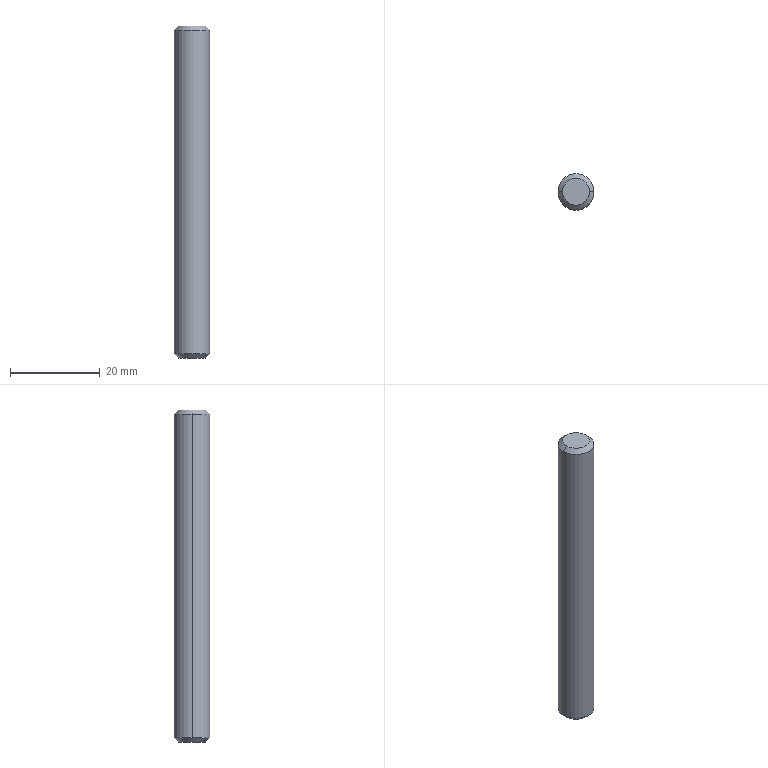Part | STEP file | BPSP-11-15 10Rotating Shaft_Default | 1 solid | 8 faces | box 8 x 8 x 74 mm | volume 3697 mm3 | cone 4 | cylinder 2 | plane 2 | commonest cylinder face diameters 8 x2
STEP:
#1=CARTESIAN_POINT('',(0.,0.,0.));
#2=DIRECTION('',(0.,0.,1.));
#3=DIRECTION('',(1.,0.,0.));
#4=AXIS2_PLACEMENT_3D('',#1,#2,#3);
#5=CARTESIAN_POINT('',(-3.,0.,-74.));
#6=VERTEX_POINT('',#5);
#7=CARTESIAN_POINT('',(3.,0.,-74.));
#8=VERTEX_POINT('',#7);
#9=CARTESIAN_POINT('',(0.,0.,-74.));
#10=DIRECTION('',(0.,0.,-1.));
#11=DIRECTION('',(1.,0.,0.));
#12=AXIS2_PLACEMENT_3D('',#9,#10,#11);
#13=CIRCLE('',#12,3.);
#14=CARTESIAN_POINT('',(0.,0.,-73.));
#15=DIRECTION('',(0.,0.,1.));
#16=DIRECTION('',(1.,0.,0.));
#17=AXIS2_PLACEMENT_3D('',#14,#15,#16);
#18=CONICAL_SURFACE('',#17,4.,0.7854);
#19=CARTESIAN_POINT('',(6.283,-1.));
#20=DIRECTION('',(-1.,0.));
#21=VECTOR('',#20,1.);
#22=LINE('',#19,#21);
#23=(GEOMETRIC_REPRESENTATION_CONTEXT(2)PARAMETRIC_REPRESENTATION_CONTEXT()REPRESENTATION_CONTEXT('',''));
#24=DEFINITIONAL_REPRESENTATION('',(#22),#23);
#25=PCURVE('',#18,#24);
#26=CARTESIAN_POINT('',(0.,0.,-74.));
#27=DIRECTION('',(0.,0.,1.));
#28=DIRECTION('',(1.,0.,0.));
#29=AXIS2_PLACEMENT_3D('',#26,#27,#28);
#30=PLANE('',#29);
#31=CARTESIAN_POINT('',(3.,0.));
#32=CARTESIAN_POINT('',(3.,-5.196));
#33=CARTESIAN_POINT('',(-1.5,-2.598));
#34=CARTESIAN_POINT('',(-6.,0.));
#35=CARTESIAN_POINT('',(-1.5,2.598));
#36=CARTESIAN_POINT('',(3.,5.196));
#37=CARTESIAN_POINT('',(3.,0.));
#38=(BOUNDED_CURVE()B_SPLINE_CURVE(2,(#31,#32,#33,#34,#35,#36,#37),.UNSPECIFIED.,.T.,.F.)B_SPLINE_CURVE_WITH_KNOTS((1,2,2,2,2,1),(-2.094,0.,2.094,4.189,6.283,8.378),.UNSPECIFIED.)CURVE()GEOMETRIC_REPRESENTATION_ITEM()RATIONAL_B_SPLINE_CURVE((1.,0.5,1.,0.5,1.,0.5,1.))REPRESENTATION_ITEM(''));
#39=(GEOMETRIC_REPRESENTATION_CONTEXT(2)PARAMETRIC_REPRESENTATION_CONTEXT()REPRESENTATION_CONTEXT('',''));
#40=DEFINITIONAL_REPRESENTATION('',(#38),#39);
#41=PCURVE('',#30,#40);
#42=SURFACE_CURVE('',#13,(#25,#41),.PCURVE_S1.);
#43=EDGE_CURVE('',#6,#8,#42,.T.);
#44=ORIENTED_EDGE('',*,*,#43,.F.);
#45=CARTESIAN_POINT('',(-4.,0.,-73.));
#46=VERTEX_POINT('',#45);
#47=CARTESIAN_POINT('',(-4.,0.,-73.));
#48=DIRECTION('',(-0.7071,0.,0.7071));
#49=VECTOR('',#48,1.);
#50=LINE('',#47,#49);
#51=CARTESIAN_POINT('',(3.142,0.));
#52=DIRECTION('',(0.,1.));
#53=VECTOR('',#52,1.);
#54=LINE('',#51,#53);
#55=(GEOMETRIC_REPRESENTATION_CONTEXT(2)PARAMETRIC_REPRESENTATION_CONTEXT()REPRESENTATION_CONTEXT('',''));
#56=DEFINITIONAL_REPRESENTATION('',(#54),#55);
#57=PCURVE('',#18,#56);
#58=CARTESIAN_POINT('',(0.,0.,-73.));
#59=DIRECTION('',(0.,0.,1.));
#60=DIRECTION('',(1.,0.,0.));
#61=AXIS2_PLACEMENT_3D('',#58,#59,#60);
#62=CONICAL_SURFACE('',#61,4.,0.7854);
#63=CARTESIAN_POINT('',(3.142,0.));
#64=DIRECTION('',(0.,1.));
#65=VECTOR('',#64,1.);
#66=LINE('',#63,#65);
#67=(GEOMETRIC_REPRESENTATION_CONTEXT(2)PARAMETRIC_REPRESENTATION_CONTEXT()REPRESENTATION_CONTEXT('',''));
#68=DEFINITIONAL_REPRESENTATION('',(#66),#67);
#69=PCURVE('',#62,#68);
#70=SURFACE_CURVE('',#50,(#57,#69),.PCURVE_S1.);
#71=EDGE_CURVE('',#6,#46,#70,.T.);
#72=ORIENTED_EDGE('',*,*,#71,.T.);
#73=CARTESIAN_POINT('',(4.,0.,-73.));
#74=VERTEX_POINT('',#73);
#75=CARTESIAN_POINT('',(0.,0.,-73.));
#76=DIRECTION('',(0.,0.,1.));
#77=DIRECTION('',(1.,0.,0.));
#78=AXIS2_PLACEMENT_3D('',#75,#76,#77);
#79=CIRCLE('',#78,4.);
#80=CARTESIAN_POINT('',(0.,0.));
#81=DIRECTION('',(1.,0.));
#82=VECTOR('',#81,1.);
#83=LINE('',#80,#82);
#84=(GEOMETRIC_REPRESENTATION_CONTEXT(2)PARAMETRIC_REPRESENTATION_CONTEXT()REPRESENTATION_CONTEXT('',''));
#85=DEFINITIONAL_REPRESENTATION('',(#83),#84);
#86=PCURVE('',#18,#85);
#87=CARTESIAN_POINT('',(0.,0.,-74.));
#88=DIRECTION('',(0.,0.,1.));
#89=DIRECTION('',(1.,0.,0.));
#90=AXIS2_PLACEMENT_3D('',#87,#88,#89);
#91=CYLINDRICAL_SURFACE('',#90,4.);
#92=CARTESIAN_POINT('',(0.,1.));
#93=DIRECTION('',(1.,0.));
#94=VECTOR('',#93,1.);
#95=LINE('',#92,#94);
#96=(GEOMETRIC_REPRESENTATION_CONTEXT(2)PARAMETRIC_REPRESENTATION_CONTEXT()REPRESENTATION_CONTEXT('',''));
#97=DEFINITIONAL_REPRESENTATION('',(#95),#96);
#98=PCURVE('',#91,#97);
#99=SURFACE_CURVE('',#79,(#86,#98),.PCURVE_S1.);
#100=EDGE_CURVE('',#74,#46,#99,.T.);
#101=ORIENTED_EDGE('',*,*,#100,.F.);
#102=CARTESIAN_POINT('',(4.,0.,-73.));
#103=DIRECTION('',(0.7071,0.,0.7071));
#104=VECTOR('',#103,1.);
#105=LINE('',#102,#104);
#106=CARTESIAN_POINT('',(0.,0.));
#107=DIRECTION('',(0.,1.));
#108=VECTOR('',#107,1.);
#109=LINE('',#106,#108);
#110=(GEOMETRIC_REPRESENTATION_CONTEXT(2)PARAMETRIC_REPRESENTATION_CONTEXT()REPRESENTATION_CONTEXT('',''));
#111=DEFINITIONAL_REPRESENTATION('',(#109),#110);
#112=PCURVE('',#18,#111);
#113=CARTESIAN_POINT('',(6.283,0.));
#114=DIRECTION('',(0.,1.));
#115=VECTOR('',#114,1.);
#116=LINE('',#113,#115);
#117=(GEOMETRIC_REPRESENTATION_CONTEXT(2)PARAMETRIC_REPRESENTATION_CONTEXT()REPRESENTATION_CONTEXT('',''));
#118=DEFINITIONAL_REPRESENTATION('',(#116),#117);
#119=PCURVE('',#62,#118);
#120=SURFACE_CURVE('',#105,(#112,#119),.PCURVE_S1.);
#121=EDGE_CURVE('',#8,#74,#120,.T.);
#122=ORIENTED_EDGE('',*,*,#121,.F.);
#123=EDGE_LOOP('',(#44,#72,#101,#122));
#124=FACE_BOUND('',#123,.T.);
#125=ADVANCED_FACE('',(#124),#18,.T.);
#126=CARTESIAN_POINT('',(3.,0.,0.));
#127=VERTEX_POINT('',#126);
#128=CARTESIAN_POINT('',(-3.,0.,0.));
#129=VERTEX_POINT('',#128);
#130=CARTESIAN_POINT('',(0.,0.,0.));
#131=DIRECTION('',(0.,0.,1.));
#132=DIRECTION('',(1.,0.,0.));
#133=AXIS2_PLACEMENT_3D('',#130,#131,#132);
#134=CIRCLE('',#133,3.);
#135=CARTESIAN_POINT('',(0.,0.,0.));
#136=DIRECTION('',(0.,0.,-1.));
#137=DIRECTION('',(-1.,0.,0.));
#138=AXIS2_PLACEMENT_3D('',#135,#136,#137);
#139=CONICAL_SURFACE('',#138,3.,0.7854);
#140=CARTESIAN_POINT('',(3.142,0.));
#141=DIRECTION('',(-1.,0.));
#142=VECTOR('',#141,1.);
#143=LINE('',#140,#142);
#144=(GEOMETRIC_REPRESENTATION_CONTEXT(2)PARAMETRIC_REPRESENTATION_CONTEXT()REPRESENTATION_CONTEXT('',''));
#145=DEFINITIONAL_REPRESENTATION('',(#143),#144);
#146=PCURVE('',#139,#145);
#147=CARTESIAN_POINT('',(0.,0.,0.));
#148=DIRECTION('',(0.,0.,1.));
#149=DIRECTION('',(1.,0.,0.));
#150=AXIS2_PLACEMENT_3D('',#147,#148,#149);
#151=PLANE('',#150);
#152=CARTESIAN_POINT('',(0.,0.));
#153=DIRECTION('',(1.,0.));
#154=AXIS2_PLACEMENT_2D('',#152,#153);
#155=CIRCLE('',#154,3.);
#156=(GEOMETRIC_REPRESENTATION_CONTEXT(2)PARAMETRIC_REPRESENTATION_CONTEXT()REPRESENTATION_CONTEXT('',''));
#157=DEFINITIONAL_REPRESENTATION('',(#155),#156);
#158=PCURVE('',#151,#157);
#159=SURFACE_CURVE('',#134,(#146,#158),.PCURVE_S1.);
#160=EDGE_CURVE('',#127,#129,#159,.T.);
#161=ORIENTED_EDGE('',*,*,#160,.F.);
#162=CARTESIAN_POINT('',(4.,0.,-1.));
#163=VERTEX_POINT('',#162);
#164=CARTESIAN_POINT('',(3.,0.,0.));
#165=DIRECTION('',(0.7071,0.,-0.7071));
#166=VECTOR('',#165,1.);
#167=LINE('',#164,#166);
#168=CARTESIAN_POINT('',(3.142,0.));
#169=DIRECTION('',(0.,1.));
#170=VECTOR('',#169,1.);
#171=LINE('',#168,#170);
#172=(GEOMETRIC_REPRESENTATION_CONTEXT(2)PARAMETRIC_REPRESENTATION_CONTEXT()REPRESENTATION_CONTEXT('',''));
#173=DEFINITIONAL_REPRESENTATION('',(#171),#172);
#174=PCURVE('',#139,#173);
#175=CARTESIAN_POINT('',(0.,0.,0.));
#176=DIRECTION('',(0.,0.,-1.));
#177=DIRECTION('',(-1.,0.,0.));
#178=AXIS2_PLACEMENT_3D('',#175,#176,#177);
#179=CONICAL_SURFACE('',#178,3.,0.7854);
#180=CARTESIAN_POINT('',(3.142,0.));
#181=DIRECTION('',(0.,1.));
#182=VECTOR('',#181,1.);
#183=LINE('',#180,#182);
#184=(GEOMETRIC_REPRESENTATION_CONTEXT(2)PARAMETRIC_REPRESENTATION_CONTEXT()REPRESENTATION_CONTEXT('',''));
#185=DEFINITIONAL_REPRESENTATION('',(#183),#184);
#186=PCURVE('',#179,#185);
#187=SURFACE_CURVE('',#167,(#174,#186),.PCURVE_S1.);
#188=EDGE_CURVE('',#127,#163,#187,.T.);
#189=ORIENTED_EDGE('',*,*,#188,.T.);
#190=CARTESIAN_POINT('',(-4.,0.,-1.));
#191=VERTEX_POINT('',#190);
#192=CARTESIAN_POINT('',(0.,0.,-1.));
#193=DIRECTION('',(0.,0.,-1.));
#194=DIRECTION('',(1.,0.,0.));
#195=AXIS2_PLACEMENT_3D('',#192,#193,#194);
#196=CIRCLE('',#195,4.);
#197=CARTESIAN_POINT('',(-3.142,1.));
#198=DIRECTION('',(1.,0.));
#199=VECTOR('',#198,1.);
#200=LINE('',#197,#199);
#201=(GEOMETRIC_REPRESENTATION_CONTEXT(2)PARAMETRIC_REPRESENTATION_CONTEXT()REPRESENTATION_CONTEXT('',''));
#202=DEFINITIONAL_REPRESENTATION('',(#200),#201);
#203=PCURVE('',#139,#202);
#204=CARTESIAN_POINT('',(6.283,73.));
#205=DIRECTION('',(-1.,0.));
#206=VECTOR('',#205,1.);
#207=LINE('',#204,#206);
#208=(GEOMETRIC_REPRESENTATION_CONTEXT(2)PARAMETRIC_REPRESENTATION_CONTEXT()REPRESENTATION_CONTEXT('',''));
#209=DEFINITIONAL_REPRESENTATION('',(#207),#208);
#210=PCURVE('',#91,#209);
#211=SURFACE_CURVE('',#196,(#203,#210),.PCURVE_S1.);
#212=EDGE_CURVE('',#191,#163,#211,.T.);
#213=ORIENTED_EDGE('',*,*,#212,.F.);
#214=CARTESIAN_POINT('',(-3.,0.,0.));
#215=DIRECTION('',(-0.7071,0.,-0.7071));
#216=VECTOR('',#215,1.);
#217=LINE('',#214,#216);
#218=CARTESIAN_POINT('',(0.,0.));
#219=DIRECTION('',(0.,1.));
#220=VECTOR('',#219,1.);
#221=LINE('',#218,#220);
#222=(GEOMETRIC_REPRESENTATION_CONTEXT(2)PARAMETRIC_REPRESENTATION_CONTEXT()REPRESENTATION_CONTEXT('',''));
#223=DEFINITIONAL_REPRESENTATION('',(#221),#222);
#224=PCURVE('',#139,#223);
#225=CARTESIAN_POINT('',(6.283,0.));
#226=DIRECTION('',(0.,1.));
#227=VECTOR('',#226,1.);
#228=LINE('',#225,#227);
#229=(GEOMETRIC_REPRESENTATION_CONTEXT(2)PARAMETRIC_REPRESENTATION_CONTEXT()REPRESENTATION_CONTEXT('',''));
#230=DEFINITIONAL_REPRESENTATION('',(#228),#229);
#231=PCURVE('',#179,#230);
#232=SURFACE_CURVE('',#217,(#224,#231),.PCURVE_S1.);
#233=EDGE_CURVE('',#129,#191,#232,.T.);
#234=ORIENTED_EDGE('',*,*,#233,.F.);
#235=EDGE_LOOP('',(#161,#189,#213,#234));
#236=FACE_BOUND('',#235,.T.);
#237=ADVANCED_FACE('',(#236),#139,.T.);
#238=ORIENTED_EDGE('',*,*,#100,.T.);
#239=CARTESIAN_POINT('',(-4.,0.,-74.));
#240=DIRECTION('',(0.,0.,1.));
#241=VECTOR('',#240,1.);
#242=LINE('',#239,#241);
#243=CARTESIAN_POINT('',(3.142,0.));
#244=DIRECTION('',(0.,1.));
#245=VECTOR('',#244,1.);
#246=LINE('',#243,#245);
#247=(GEOMETRIC_REPRESENTATION_CONTEXT(2)PARAMETRIC_REPRESENTATION_CONTEXT()REPRESENTATION_CONTEXT('',''));
#248=DEFINITIONAL_REPRESENTATION('',(#246),#247);
#249=PCURVE('',#91,#248);
#250=CARTESIAN_POINT('',(0.,0.,-74.));
#251=DIRECTION('',(0.,0.,1.));
#252=DIRECTION('',(1.,0.,0.));
#253=AXIS2_PLACEMENT_3D('',#250,#251,#252);
#254=CYLINDRICAL_SURFACE('',#253,4.);
#255=CARTESIAN_POINT('',(3.142,0.));
#256=DIRECTION('',(0.,1.));
#257=VECTOR('',#256,1.);
#258=LINE('',#255,#257);
#259=(GEOMETRIC_REPRESENTATION_CONTEXT(2)PARAMETRIC_REPRESENTATION_CONTEXT()REPRESENTATION_CONTEXT('',''));
#260=DEFINITIONAL_REPRESENTATION('',(#258),#259);
#261=PCURVE('',#254,#260);
#262=SURFACE_CURVE('',#242,(#249,#261),.PCURVE_S1.);
#263=EDGE_CURVE('',#46,#191,#262,.T.);
#264=ORIENTED_EDGE('',*,*,#263,.T.);
#265=ORIENTED_EDGE('',*,*,#212,.T.);
#266=CARTESIAN_POINT('',(4.,0.,-74.));
#267=DIRECTION('',(0.,0.,1.));
#268=VECTOR('',#267,1.);
#269=LINE('',#266,#268);
#270=CARTESIAN_POINT('',(0.,0.));
#271=DIRECTION('',(0.,1.));
#272=VECTOR('',#271,1.);
#273=LINE('',#270,#272);
#274=(GEOMETRIC_REPRESENTATION_CONTEXT(2)PARAMETRIC_REPRESENTATION_CONTEXT()REPRESENTATION_CONTEXT('',''));
#275=DEFINITIONAL_REPRESENTATION('',(#273),#274);
#276=PCURVE('',#91,#275);
#277=CARTESIAN_POINT('',(6.283,0.));
#278=DIRECTION('',(0.,1.));
#279=VECTOR('',#278,1.);
#280=LINE('',#277,#279);
#281=(GEOMETRIC_REPRESENTATION_CONTEXT(2)PARAMETRIC_REPRESENTATION_CONTEXT()REPRESENTATION_CONTEXT('',''));
#282=DEFINITIONAL_REPRESENTATION('',(#280),#281);
#283=PCURVE('',#254,#282);
#284=SURFACE_CURVE('',#269,(#276,#283),.PCURVE_S1.);
#285=EDGE_CURVE('',#74,#163,#284,.T.);
#286=ORIENTED_EDGE('',*,*,#285,.F.);
#287=EDGE_LOOP('',(#238,#264,#265,#286));
#288=FACE_BOUND('',#287,.T.);
#289=ADVANCED_FACE('',(#288),#91,.T.);
#290=ORIENTED_EDGE('',*,*,#263,.F.);
#291=CARTESIAN_POINT('',(0.,0.,-73.));
#292=DIRECTION('',(0.,0.,1.));
#293=DIRECTION('',(1.,0.,0.));
#294=AXIS2_PLACEMENT_3D('',#291,#292,#293);
#295=CIRCLE('',#294,4.);
#296=CARTESIAN_POINT('',(0.,1.));
#297=DIRECTION('',(1.,0.));
#298=VECTOR('',#297,1.);
#299=LINE('',#296,#298);
#300=(GEOMETRIC_REPRESENTATION_CONTEXT(2)PARAMETRIC_REPRESENTATION_CONTEXT()REPRESENTATION_CONTEXT('',''));
#301=DEFINITIONAL_REPRESENTATION('',(#299),#300);
#302=PCURVE('',#254,#301);
#303=CARTESIAN_POINT('',(0.,0.));
#304=DIRECTION('',(1.,0.));
#305=VECTOR('',#304,1.);
#306=LINE('',#303,#305);
#307=(GEOMETRIC_REPRESENTATION_CONTEXT(2)PARAMETRIC_REPRESENTATION_CONTEXT()REPRESENTATION_CONTEXT('',''));
#308=DEFINITIONAL_REPRESENTATION('',(#306),#307);
#309=PCURVE('',#62,#308);
#310=SURFACE_CURVE('',#295,(#302,#309),.PCURVE_S1.);
#311=EDGE_CURVE('',#46,#74,#310,.T.);
#312=ORIENTED_EDGE('',*,*,#311,.T.);
#313=ORIENTED_EDGE('',*,*,#285,.T.);
#314=CARTESIAN_POINT('',(0.,0.,-1.));
#315=DIRECTION('',(0.,0.,-1.));
#316=DIRECTION('',(1.,0.,0.));
#317=AXIS2_PLACEMENT_3D('',#314,#315,#316);
#318=CIRCLE('',#317,4.);
#319=CARTESIAN_POINT('',(6.283,73.));
#320=DIRECTION('',(-1.,0.));
#321=VECTOR('',#320,1.);
#322=LINE('',#319,#321);
#323=(GEOMETRIC_REPRESENTATION_CONTEXT(2)PARAMETRIC_REPRESENTATION_CONTEXT()REPRESENTATION_CONTEXT('',''));
#324=DEFINITIONAL_REPRESENTATION('',(#322),#323);
#325=PCURVE('',#254,#324);
#326=CARTESIAN_POINT('',(3.142,1.));
#327=DIRECTION('',(1.,0.));
#328=VECTOR('',#327,1.);
#329=LINE('',#326,#328);
#330=(GEOMETRIC_REPRESENTATION_CONTEXT(2)PARAMETRIC_REPRESENTATION_CONTEXT()REPRESENTATION_CONTEXT('',''));
#331=DEFINITIONAL_REPRESENTATION('',(#329),#330);
#332=PCURVE('',#179,#331);
#333=SURFACE_CURVE('',#318,(#325,#332),.PCURVE_S1.);
#334=EDGE_CURVE('',#163,#191,#333,.T.);
#335=ORIENTED_EDGE('',*,*,#334,.T.);
#336=EDGE_LOOP('',(#290,#312,#313,#335));
#337=FACE_BOUND('',#336,.T.);
#338=ADVANCED_FACE('',(#337),#254,.T.);
#339=CARTESIAN_POINT('',(0.,0.,-74.));
#340=DIRECTION('',(0.,0.,-1.));
#341=DIRECTION('',(1.,0.,0.));
#342=AXIS2_PLACEMENT_3D('',#339,#340,#341);
#343=CIRCLE('',#342,3.);
#344=CARTESIAN_POINT('',(3.,0.));
#345=CARTESIAN_POINT('',(3.,-5.196));
#346=CARTESIAN_POINT('',(-1.5,-2.598));
#347=CARTESIAN_POINT('',(-6.,0.));
#348=CARTESIAN_POINT('',(-1.5,2.598));
#349=CARTESIAN_POINT('',(3.,5.196));
#350=CARTESIAN_POINT('',(3.,0.));
#351=(BOUNDED_CURVE()B_SPLINE_CURVE(2,(#344,#345,#346,#347,#348,#349,#350),.UNSPECIFIED.,.T.,.F.)B_SPLINE_CURVE_WITH_KNOTS((1,2,2,2,2,1),(-2.094,0.,2.094,4.189,6.283,8.378),.UNSPECIFIED.)CURVE()GEOMETRIC_REPRESENTATION_ITEM()RATIONAL_B_SPLINE_CURVE((1.,0.5,1.,0.5,1.,0.5,1.))REPRESENTATION_ITEM(''));
#352=(GEOMETRIC_REPRESENTATION_CONTEXT(2)PARAMETRIC_REPRESENTATION_CONTEXT()REPRESENTATION_CONTEXT('',''));
#353=DEFINITIONAL_REPRESENTATION('',(#351),#352);
#354=PCURVE('',#30,#353);
#355=CARTESIAN_POINT('',(6.283,-1.));
#356=DIRECTION('',(-1.,0.));
#357=VECTOR('',#356,1.);
#358=LINE('',#355,#357);
#359=(GEOMETRIC_REPRESENTATION_CONTEXT(2)PARAMETRIC_REPRESENTATION_CONTEXT()REPRESENTATION_CONTEXT('',''));
#360=DEFINITIONAL_REPRESENTATION('',(#358),#359);
#361=PCURVE('',#62,#360);
#362=SURFACE_CURVE('',#343,(#354,#361),.PCURVE_S1.);
#363=EDGE_CURVE('',#8,#6,#362,.T.);
#364=ORIENTED_EDGE('',*,*,#363,.T.);
#365=ORIENTED_EDGE('',*,*,#43,.T.);
#366=EDGE_LOOP('',(#364,#365));
#367=FACE_BOUND('',#366,.T.);
#368=ADVANCED_FACE('',(#367),#30,.F.);
#369=CARTESIAN_POINT('',(0.,0.,0.));
#370=DIRECTION('',(0.,0.,1.));
#371=DIRECTION('',(1.,0.,0.));
#372=AXIS2_PLACEMENT_3D('',#369,#370,#371);
#373=CIRCLE('',#372,3.);
#374=CARTESIAN_POINT('',(0.,0.));
#375=DIRECTION('',(1.,0.));
#376=AXIS2_PLACEMENT_2D('',#374,#375);
#377=CIRCLE('',#376,3.);
#378=(GEOMETRIC_REPRESENTATION_CONTEXT(2)PARAMETRIC_REPRESENTATION_CONTEXT()REPRESENTATION_CONTEXT('',''));
#379=DEFINITIONAL_REPRESENTATION('',(#377),#378);
#380=PCURVE('',#151,#379);
#381=CARTESIAN_POINT('',(9.425,0.));
#382=DIRECTION('',(-1.,0.));
#383=VECTOR('',#382,1.);
#384=LINE('',#381,#383);
#385=(GEOMETRIC_REPRESENTATION_CONTEXT(2)PARAMETRIC_REPRESENTATION_CONTEXT()REPRESENTATION_CONTEXT('',''));
#386=DEFINITIONAL_REPRESENTATION('',(#384),#385);
#387=PCURVE('',#179,#386);
#388=SURFACE_CURVE('',#373,(#380,#387),.PCURVE_S1.);
#389=EDGE_CURVE('',#129,#127,#388,.T.);
#390=ORIENTED_EDGE('',*,*,#389,.T.);
#391=ORIENTED_EDGE('',*,*,#160,.T.);
#392=EDGE_LOOP('',(#390,#391));
#393=FACE_BOUND('',#392,.T.);
#394=ADVANCED_FACE('',(#393),#151,.T.);
#395=ORIENTED_EDGE('',*,*,#188,.F.);
#396=ORIENTED_EDGE('',*,*,#389,.F.);
#397=ORIENTED_EDGE('',*,*,#233,.T.);
#398=ORIENTED_EDGE('',*,*,#334,.F.);
#399=EDGE_LOOP('',(#395,#396,#397,#398));
#400=FACE_BOUND('',#399,.T.);
#401=ADVANCED_FACE('',(#400),#179,.T.);
#402=ORIENTED_EDGE('',*,*,#71,.F.);
#403=ORIENTED_EDGE('',*,*,#363,.F.);
#404=ORIENTED_EDGE('',*,*,#121,.T.);
#405=ORIENTED_EDGE('',*,*,#311,.F.);
#406=EDGE_LOOP('',(#402,#403,#404,#405));
#407=FACE_BOUND('',#406,.T.);
#408=ADVANCED_FACE('',(#407),#62,.T.);
#409=CLOSED_SHELL('',(#125,#237,#289,#338,#368,#394,#401,#408));
#410=MANIFOLD_SOLID_BREP('',#409);
#411=(LENGTH_UNIT()NAMED_UNIT(*)SI_UNIT(.MILLI.,.METRE.));
#412=UNCERTAINTY_MEASURE_WITH_UNIT(LENGTH_MEASURE(0.0000001),#411,'','');
#413=(NAMED_UNIT(*)PLANE_ANGLE_UNIT()SI_UNIT($,.RADIAN.));
#414=(NAMED_UNIT(*)SI_UNIT($,.STERADIAN.)SOLID_ANGLE_UNIT());
#415=(GEOMETRIC_REPRESENTATION_CONTEXT(3)GLOBAL_UNCERTAINTY_ASSIGNED_CONTEXT((#412))GLOBAL_UNIT_ASSIGNED_CONTEXT((#411,#413,#414))REPRESENTATION_CONTEXT('',''));
#416=ADVANCED_BREP_SHAPE_REPRESENTATION('',(#4,#410),#415);